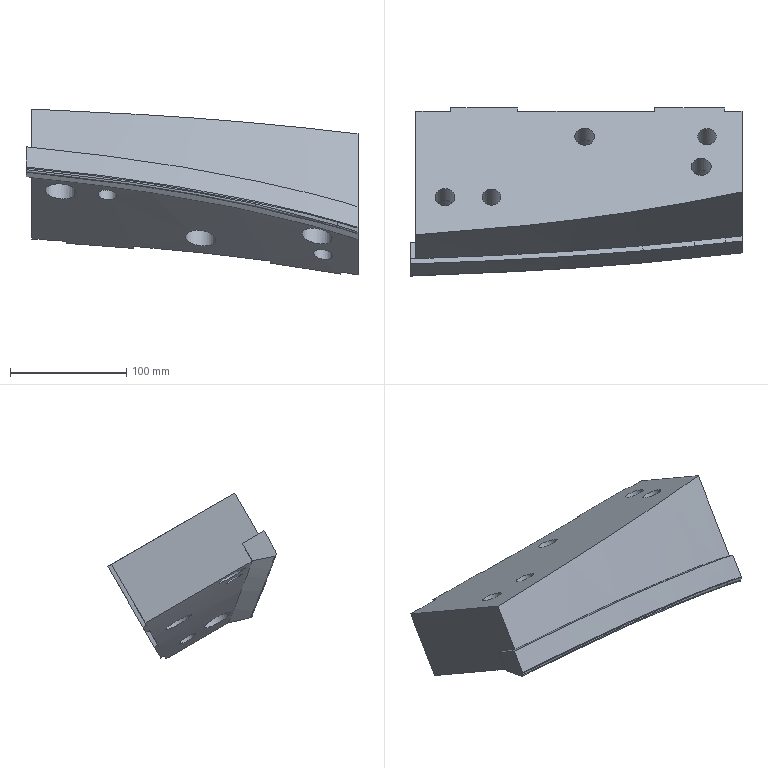Part | NX | features MAIN_BODY 2 | 1 solid | 44 faces | box 285 x 144.432 x 142.307 mm | volume 2052908 mm3 | spline 19 | plane 17 | cylinder 8 | commonest cylinder face diameters 17 x3 26 x3 16 x2